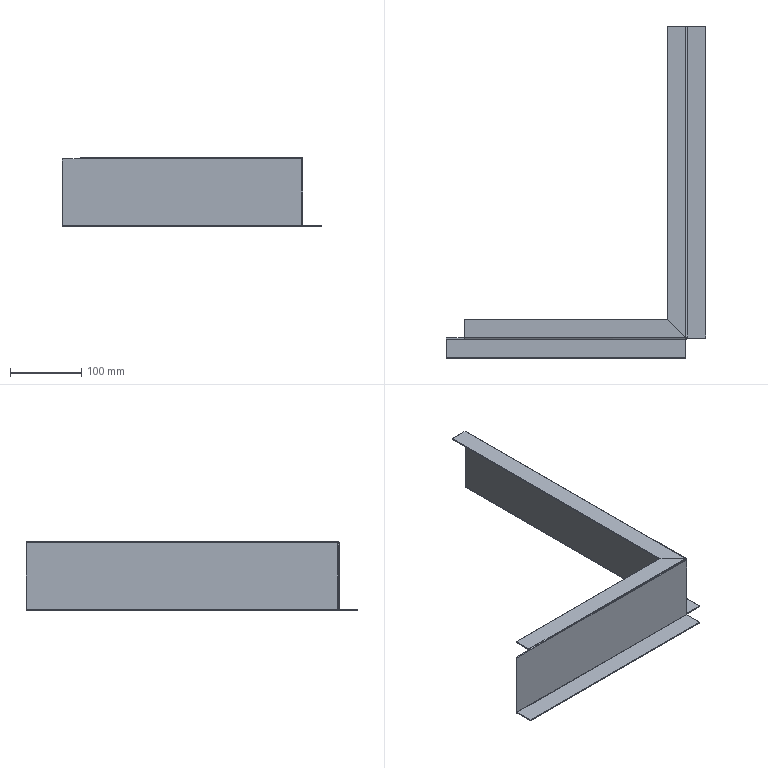Part | STEP file | HESS-408-70-15W-W-37-upper door glass inner frame 3 | 1 solid | 39 faces | box 365 x 466.5 x 97 mm | volume 170617 mm3 | plane 26 | cylinder 11 | spline 2 | commonest cylinder face diameters 0.2 x5 3.2 x5 1 x1